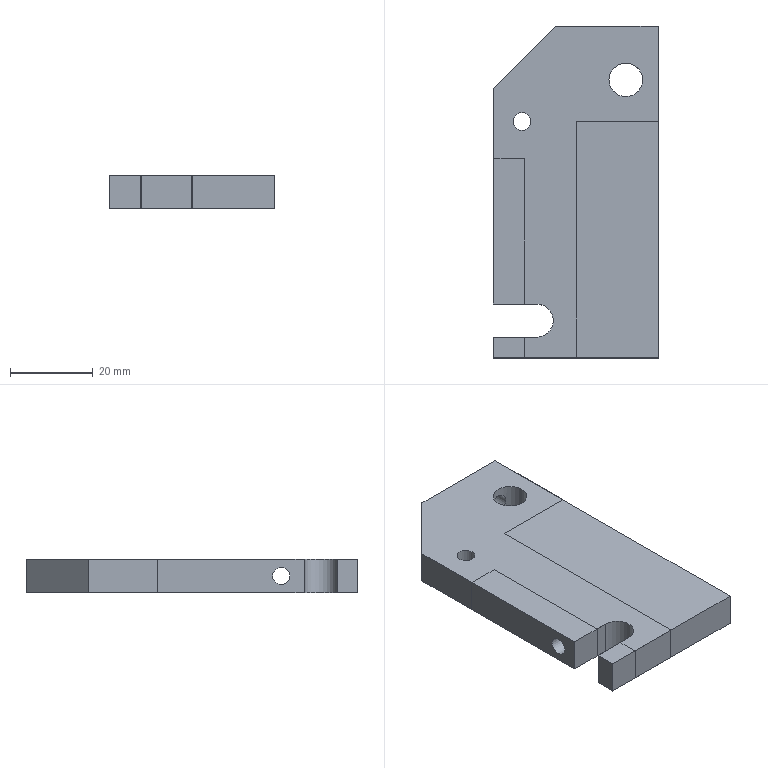NC program | NX | posted with a generic post | part box 40 x 80 x 8 mm
Whole program:
N10 G17 G21 G94 G90
(DRILLING_2 , TOOL : 倒角D10-90度)
N12 T02 M6
N14 G54
N16 G17 G0 G90 X32. Y0. B0. C0. S1200 M3
N18 G43 Z3. H2
N20 G94 G81 G99 Z-1. F60. R3.
N22 G80
N24 M5
(DRILLING_2_COPY , TOOL : 钻头D4.3-54-83)
N26 T13 M6
N28 G54
N30 G17 G0 G90 X32. Y0. B0. C0. S1300 M3
N32 G43 Z3. H13
N34 G94 G83 G99 Z-15. F60. Q2. R3.
N36 G80
N38 M5
(DRILLING_2_COPY_1 , TOOL : 倒角D10-90度)
N40 T02 M6
N42 G54
N44 G17 G0 G90 X32. Y0. B0. C0. S2000 M3
N46 G43 Z3. H2
N48 G94 G81 G99 Z-2.5 F120. R3.
N50 G80
N52 M5
(DRILLING_2_COPY_COPY , TOOL : 上排M5-22-D5.5-60)
N54 T12 M6
N56 G54
N58 G17 G0 G90 X32. Y0. B0. C0. S300 M3
N60 G43 Z3. H12
N62 G84 G94 G99 Z-5. F240. R3.
N64 G80
N66 M5
N68 M2